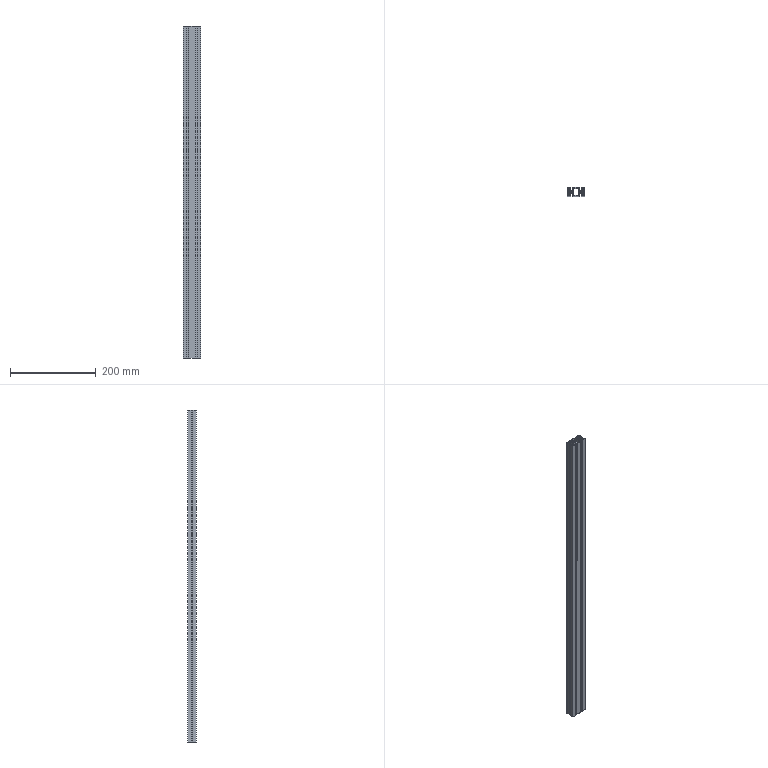Part | SolidWorks | features BaseBody 1 | 1 solid | 76 faces | box 40 x 20 x 775 mm | volume 232976 mm3 | plane 54 | cylinder 22 | commonest cylinder face diameters 10.875 x10 4 x8 3.5 x4